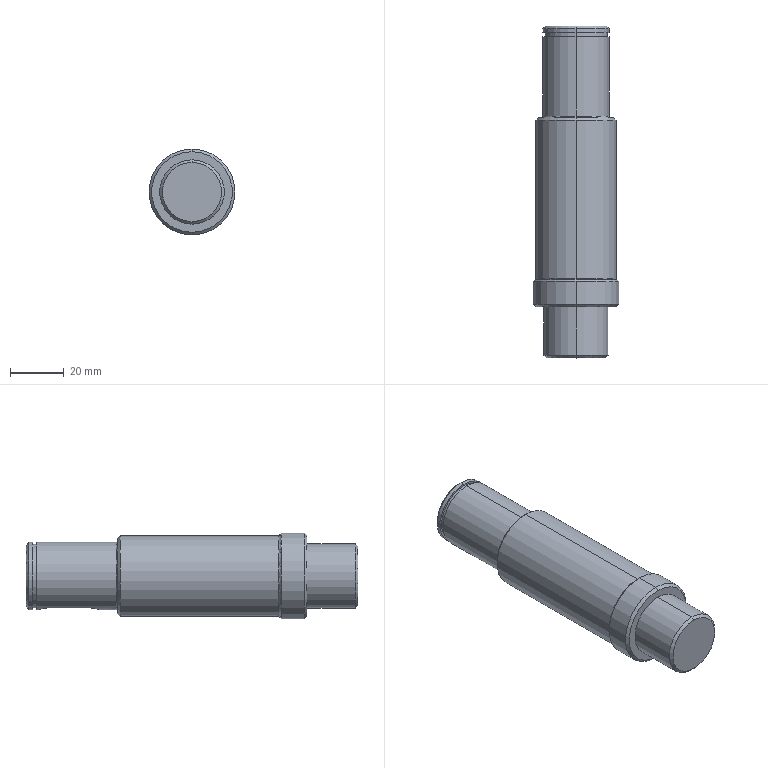Part | SolidWorks | features BaseBody 1 | 1 solid | 38 faces | box 32 x 123.5 x 32 mm | volume 75377 mm3 | cylinder 14 | cone 10 | plane 10 | spline 4 | commonest cylinder face diameters 25 x4 8 x2 23.5 x2 24 x2 30 x2 32 x2